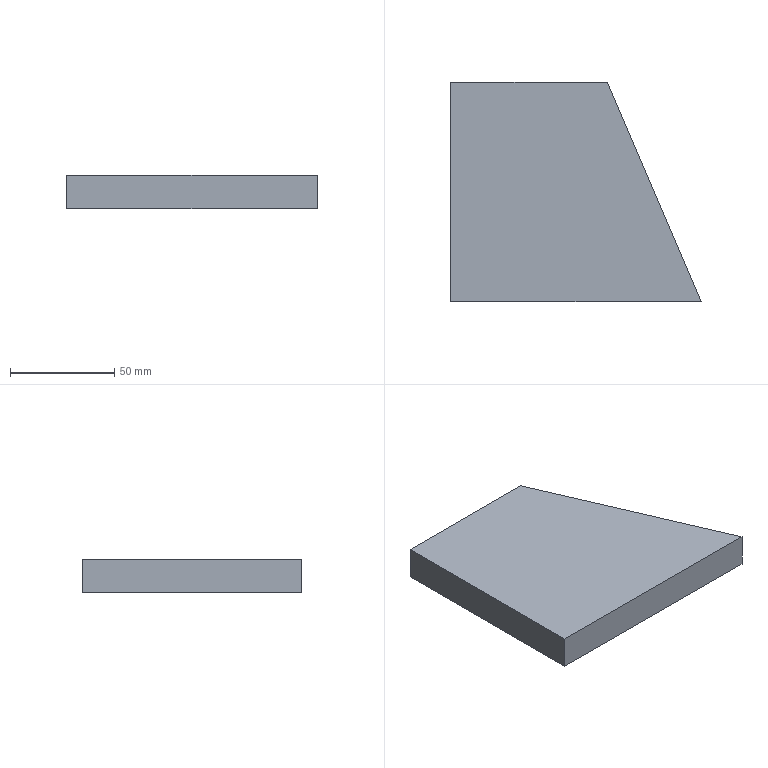Part | SolidWorks | features Extrusion 1 | 1 solid | 6 faces | box 120 x 105 x 16 mm | volume 163800 mm3 | plane 6
STEP:
#1=CARTESIAN_POINT('',(0.,0.,-8.));
#2=VERTEX_POINT('',#1);
#3=CARTESIAN_POINT('',(120.,0.,-8.));
#4=VERTEX_POINT('',#3);
#5=CARTESIAN_POINT('',(120.,0.,-8.));
#6=DIRECTION('',(1.,0.,0.));
#7=VECTOR('',#6,1000.);
#8=LINE('',#5,#7);
#9=EDGE_CURVE('',#2,#4,#8,.T.);
#10=ORIENTED_EDGE('',*,*,#9,.T.);
#11=CARTESIAN_POINT('',(120.,0.,8.));
#12=VERTEX_POINT('',#11);
#13=CARTESIAN_POINT('',(120.,0.,8.));
#14=DIRECTION('',(0.,0.,-1.));
#15=VECTOR('',#14,1000.);
#16=LINE('',#13,#15);
#17=EDGE_CURVE('',#12,#4,#16,.T.);
#18=ORIENTED_EDGE('',*,*,#17,.F.);
#19=CARTESIAN_POINT('',(0.,0.,8.));
#20=VERTEX_POINT('',#19);
#21=CARTESIAN_POINT('',(120.,0.,8.));
#22=DIRECTION('',(1.,0.,0.));
#23=VECTOR('',#22,1000.);
#24=LINE('',#21,#23);
#25=EDGE_CURVE('',#20,#12,#24,.T.);
#26=ORIENTED_EDGE('',*,*,#25,.F.);
#27=CARTESIAN_POINT('',(0.,0.,8.));
#28=DIRECTION('',(0.,0.,-1.));
#29=VECTOR('',#28,1000.);
#30=LINE('',#27,#29);
#31=EDGE_CURVE('',#20,#2,#30,.T.);
#32=ORIENTED_EDGE('',*,*,#31,.T.);
#33=EDGE_LOOP('',(#10,#18,#26,#32));
#34=FACE_OUTER_BOUND('',#33,.T.);
#35=CARTESIAN_POINT('',(120.,0.,8.));
#36=DIRECTION('',(0.,1.,0.));
#37=DIRECTION('',(-1.,0.,0.));
#38=AXIS2_PLACEMENT_3D('',#35,#36,#37);
#39=PLANE('',#38);
#40=ADVANCED_FACE('',(#34),#39,.F.);
#41=CARTESIAN_POINT('',(75.,105.,-8.));
#42=VERTEX_POINT('',#41);
#43=CARTESIAN_POINT('',(75.,105.,-8.));
#44=DIRECTION('',(-0.3939,0.9191,0.));
#45=VECTOR('',#44,1000.);
#46=LINE('',#43,#45);
#47=EDGE_CURVE('',#4,#42,#46,.T.);
#48=ORIENTED_EDGE('',*,*,#47,.T.);
#49=CARTESIAN_POINT('',(75.,105.,8.));
#50=VERTEX_POINT('',#49);
#51=CARTESIAN_POINT('',(75.,105.,8.));
#52=DIRECTION('',(0.,0.,-1.));
#53=VECTOR('',#52,1000.);
#54=LINE('',#51,#53);
#55=EDGE_CURVE('',#50,#42,#54,.T.);
#56=ORIENTED_EDGE('',*,*,#55,.F.);
#57=CARTESIAN_POINT('',(75.,105.,8.));
#58=DIRECTION('',(-0.3939,0.9191,0.));
#59=VECTOR('',#58,1000.);
#60=LINE('',#57,#59);
#61=EDGE_CURVE('',#12,#50,#60,.T.);
#62=ORIENTED_EDGE('',*,*,#61,.F.);
#63=ORIENTED_EDGE('',*,*,#17,.T.);
#64=EDGE_LOOP('',(#48,#56,#62,#63));
#65=FACE_OUTER_BOUND('',#64,.T.);
#66=CARTESIAN_POINT('',(75.,105.,8.));
#67=DIRECTION('',(-0.9191,-0.3939,0.));
#68=DIRECTION('',(0.3939,-0.9191,0.));
#69=AXIS2_PLACEMENT_3D('',#66,#67,#68);
#70=PLANE('',#69);
#71=ADVANCED_FACE('',(#65),#70,.F.);
#72=CARTESIAN_POINT('',(0.,105.,-8.));
#73=VERTEX_POINT('',#72);
#74=CARTESIAN_POINT('',(0.,105.,-8.));
#75=DIRECTION('',(-1.,0.,0.));
#76=VECTOR('',#75,1000.);
#77=LINE('',#74,#76);
#78=EDGE_CURVE('',#42,#73,#77,.T.);
#79=ORIENTED_EDGE('',*,*,#78,.T.);
#80=CARTESIAN_POINT('',(0.,105.,8.));
#81=VERTEX_POINT('',#80);
#82=CARTESIAN_POINT('',(0.,105.,8.));
#83=DIRECTION('',(0.,0.,-1.));
#84=VECTOR('',#83,1000.);
#85=LINE('',#82,#84);
#86=EDGE_CURVE('',#81,#73,#85,.T.);
#87=ORIENTED_EDGE('',*,*,#86,.F.);
#88=CARTESIAN_POINT('',(0.,105.,8.));
#89=DIRECTION('',(-1.,0.,0.));
#90=VECTOR('',#89,1000.);
#91=LINE('',#88,#90);
#92=EDGE_CURVE('',#50,#81,#91,.T.);
#93=ORIENTED_EDGE('',*,*,#92,.F.);
#94=ORIENTED_EDGE('',*,*,#55,.T.);
#95=EDGE_LOOP('',(#79,#87,#93,#94));
#96=FACE_OUTER_BOUND('',#95,.T.);
#97=CARTESIAN_POINT('',(0.,105.,8.));
#98=DIRECTION('',(0.,-1.,0.));
#99=DIRECTION('',(0.,0.,-1.));
#100=AXIS2_PLACEMENT_3D('',#97,#98,#99);
#101=PLANE('',#100);
#102=ADVANCED_FACE('',(#96),#101,.F.);
#103=CARTESIAN_POINT('',(0.,0.,-8.));
#104=DIRECTION('',(0.,-1.,0.));
#105=VECTOR('',#104,1000.);
#106=LINE('',#103,#105);
#107=EDGE_CURVE('',#73,#2,#106,.T.);
#108=ORIENTED_EDGE('',*,*,#107,.T.);
#109=ORIENTED_EDGE('',*,*,#31,.F.);
#110=CARTESIAN_POINT('',(0.,0.,8.));
#111=DIRECTION('',(0.,-1.,0.));
#112=VECTOR('',#111,1000.);
#113=LINE('',#110,#112);
#114=EDGE_CURVE('',#81,#20,#113,.T.);
#115=ORIENTED_EDGE('',*,*,#114,.F.);
#116=ORIENTED_EDGE('',*,*,#86,.T.);
#117=EDGE_LOOP('',(#108,#109,#115,#116));
#118=FACE_OUTER_BOUND('',#117,.T.);
#119=CARTESIAN_POINT('',(0.,0.,8.));
#120=DIRECTION('',(1.,0.,0.));
#121=DIRECTION('',(0.,0.,-1.));
#122=AXIS2_PLACEMENT_3D('',#119,#120,#121);
#123=PLANE('',#122);
#124=ADVANCED_FACE('',(#118),#123,.F.);
#125=ORIENTED_EDGE('',*,*,#25,.T.);
#126=ORIENTED_EDGE('',*,*,#61,.T.);
#127=ORIENTED_EDGE('',*,*,#92,.T.);
#128=ORIENTED_EDGE('',*,*,#114,.T.);
#129=EDGE_LOOP('',(#125,#126,#127,#128));
#130=FACE_OUTER_BOUND('',#129,.T.);
#131=CARTESIAN_POINT('',(0.,0.,8.));
#132=DIRECTION('',(0.,0.,-1.));
#133=DIRECTION('',(-1.,0.,0.));
#134=AXIS2_PLACEMENT_3D('',#131,#132,#133);
#135=PLANE('',#134);
#136=ADVANCED_FACE('',(#130),#135,.F.);
#137=ORIENTED_EDGE('',*,*,#9,.F.);
#138=ORIENTED_EDGE('',*,*,#107,.F.);
#139=ORIENTED_EDGE('',*,*,#78,.F.);
#140=ORIENTED_EDGE('',*,*,#47,.F.);
#141=EDGE_LOOP('',(#137,#138,#139,#140));
#142=FACE_OUTER_BOUND('',#141,.T.);
#143=CARTESIAN_POINT('',(0.,0.,-8.));
#144=DIRECTION('',(0.,0.,-1.));
#145=DIRECTION('',(-1.,0.,0.));
#146=AXIS2_PLACEMENT_3D('',#143,#144,#145);
#147=PLANE('',#146);
#148=ADVANCED_FACE('',(#142),#147,.T.);
#149=CLOSED_SHELL('',(#40,#71,#102,#124,#136,#148));
#150=MANIFOLD_SOLID_BREP('',#149);
#151=CARTESIAN_POINT('',(0.,0.,0.));
#152=DIRECTION('',(0.,0.,1.));
#153=DIRECTION('',(1.,0.,0.));
#154=AXIS2_PLACEMENT_3D('',#151,#152,#153);
#155=(LENGTH_UNIT()NAMED_UNIT(*)SI_UNIT(.MILLI.,.METRE.));
#156=UNCERTAINTY_MEASURE_WITH_UNIT(LENGTH_MEASURE(0.00001),#155,'','');
#157=(NAMED_UNIT(*)PLANE_ANGLE_UNIT()SI_UNIT($,.RADIAN.));
#158=(NAMED_UNIT(*)SI_UNIT($,.STERADIAN.)SOLID_ANGLE_UNIT());
#159=(GEOMETRIC_REPRESENTATION_CONTEXT(3)GLOBAL_UNCERTAINTY_ASSIGNED_CONTEXT((#156))GLOBAL_UNIT_ASSIGNED_CONTEXT((#155,#157,#158))REPRESENTATION_CONTEXT('',''));
#160=ADVANCED_BREP_SHAPE_REPRESENTATION('',(#150,#154),#159);